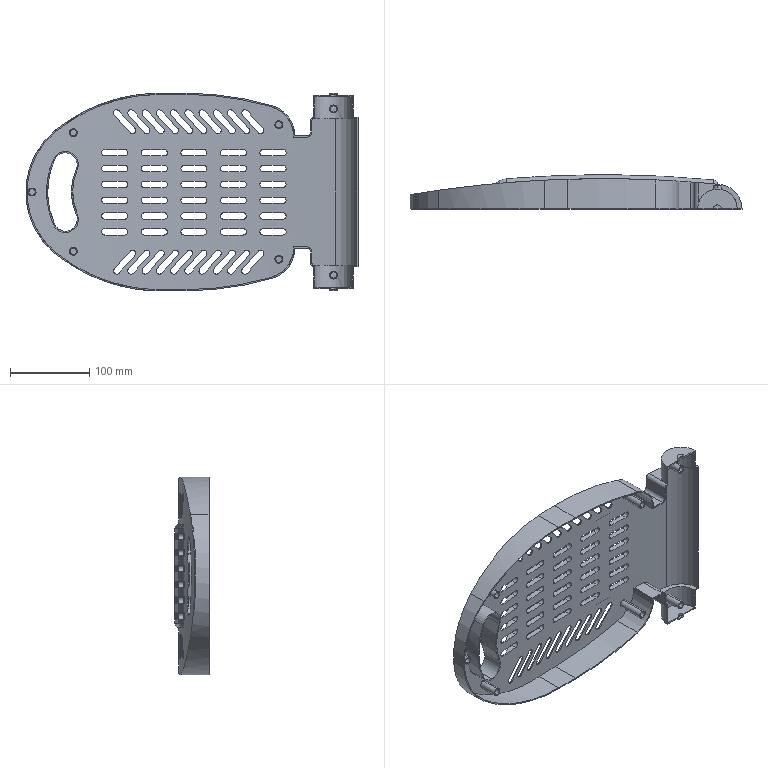Part | SolidWorks | features ICE 8, Fillet 3, CombineBodies 1, Extrusion 1, MirrorPattern 1, Shell 1 | 1 solid | 368 faces | box 420 x 43.06 x 250 mm | volume 321322 mm3 | cylinder 227 | plane 133 | torus 6 | sphere 2 | commonest cylinder face diameters 8 x138 10 x25 40 x14 2997 x8 7 x4 47 x4